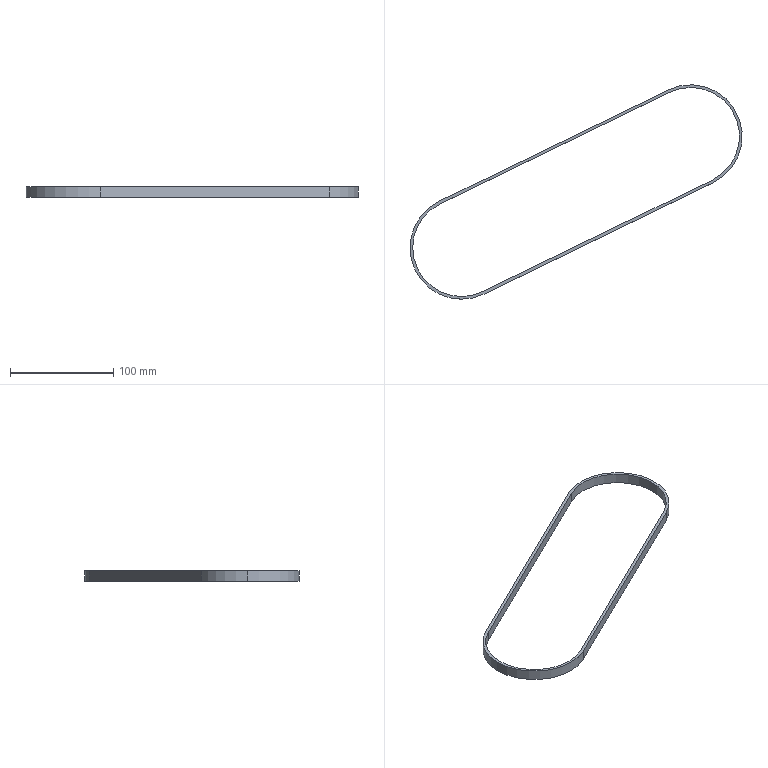Part | STEP file | Belt 1-18^ twist assembly SGN-4 | 1 solid | 12 faces | box 321.782 x 207.752 x 10 mm | volume 20933 mm3 | cylinder 6 | plane 6 | commonest cylinder face diameters 94.53 x3 99.77 x3
STEP:
#1=CARTESIAN_POINT('',(0.,0.,0.));
#2=DIRECTION('',(0.,0.,1.));
#3=DIRECTION('',(1.,0.,0.));
#4=AXIS2_PLACEMENT_3D('',#1,#2,#3);
#5=CARTESIAN_POINT('',(-141.649,-4.675,10.));
#6=VERTEX_POINT('',#5);
#7=CARTESIAN_POINT('',(-141.649,-4.675,0.));
#8=VERTEX_POINT('',#7);
#9=CARTESIAN_POINT('',(-141.649,-4.675,10.));
#10=DIRECTION('',(0.,0.,-1.));
#11=VECTOR('',#10,1.);
#12=LINE('',#9,#11);
#13=CARTESIAN_POINT('',(-120.976,-47.179,10.));
#14=DIRECTION('',(0.,0.,-1.));
#15=DIRECTION('',(-1.,0.,0.));
#16=AXIS2_PLACEMENT_3D('',#13,#14,#15);
#17=CYLINDRICAL_SURFACE('',#16,47.265);
#18=CARTESIAN_POINT('',(1.118,0.));
#19=DIRECTION('',(0.,1.));
#20=VECTOR('',#19,1.);
#21=LINE('',#18,#20);
#22=(GEOMETRIC_REPRESENTATION_CONTEXT(2)PARAMETRIC_REPRESENTATION_CONTEXT()REPRESENTATION_CONTEXT('',''));
#23=DEFINITIONAL_REPRESENTATION('',(#21),#22);
#24=PCURVE('',#17,#23);
#25=CARTESIAN_POINT('',(-141.649,-4.675,10.));
#26=DIRECTION('',(0.4374,-0.8993,0.));
#27=DIRECTION('',(0.8993,0.4374,0.));
#28=AXIS2_PLACEMENT_3D('',#25,#26,#27);
#29=PLANE('',#28);
#30=CARTESIAN_POINT('',(0.,0.));
#31=DIRECTION('',(0.,-1.));
#32=VECTOR('',#31,1.);
#33=LINE('',#30,#32);
#34=(GEOMETRIC_REPRESENTATION_CONTEXT(2)PARAMETRIC_REPRESENTATION_CONTEXT()REPRESENTATION_CONTEXT('',''));
#35=DEFINITIONAL_REPRESENTATION('',(#33),#34);
#36=PCURVE('',#29,#35);
#37=SURFACE_CURVE('',#12,(#24,#36),.PCURVE_S1.);
#38=EDGE_CURVE('',#6,#8,#37,.T.);
#39=ORIENTED_EDGE('',*,*,#38,.T.);
#40=CARTESIAN_POINT('',(-168.241,-47.179,0.));
#41=VERTEX_POINT('',#40);
#42=CARTESIAN_POINT('',(-120.976,-47.179,0.));
#43=DIRECTION('',(0.,0.,1.));
#44=DIRECTION('',(-1.,0.,0.));
#45=AXIS2_PLACEMENT_3D('',#42,#43,#44);
#46=CIRCLE('',#45,47.265);
#47=CARTESIAN_POINT('',(6.283,10.));
#48=DIRECTION('',(-1.,0.));
#49=VECTOR('',#48,1.);
#50=LINE('',#47,#49);
#51=(GEOMETRIC_REPRESENTATION_CONTEXT(2)PARAMETRIC_REPRESENTATION_CONTEXT()REPRESENTATION_CONTEXT('',''));
#52=DEFINITIONAL_REPRESENTATION('',(#50),#51);
#53=PCURVE('',#17,#52);
#54=CARTESIAN_POINT('',(-120.976,-47.179,0.));
#55=DIRECTION('',(0.,0.,-1.));
#56=DIRECTION('',(-1.,0.,0.));
#57=AXIS2_PLACEMENT_3D('',#54,#55,#56);
#58=PLANE('',#57);
#59=CARTESIAN_POINT('',(47.265,0.));
#60=CARTESIAN_POINT('',(47.265,-81.865));
#61=CARTESIAN_POINT('',(-23.633,-40.933));
#62=CARTESIAN_POINT('',(-94.53,0.));
#63=CARTESIAN_POINT('',(-23.633,40.933));
#64=CARTESIAN_POINT('',(47.265,81.865));
#65=CARTESIAN_POINT('',(47.265,0.));
#66=(BOUNDED_CURVE()B_SPLINE_CURVE(2,(#59,#60,#61,#62,#63,#64,#65),.UNSPECIFIED.,.T.,.F.)B_SPLINE_CURVE_WITH_KNOTS((1,2,2,2,2,1),(-2.094,0.,2.094,4.189,6.283,8.378),.UNSPECIFIED.)CURVE()GEOMETRIC_REPRESENTATION_ITEM()RATIONAL_B_SPLINE_CURVE((1.,0.5,1.,0.5,1.,0.5,1.))REPRESENTATION_ITEM(''));
#67=(GEOMETRIC_REPRESENTATION_CONTEXT(2)PARAMETRIC_REPRESENTATION_CONTEXT()REPRESENTATION_CONTEXT('',''));
#68=DEFINITIONAL_REPRESENTATION('',(#66),#67);
#69=PCURVE('',#58,#68);
#70=SURFACE_CURVE('',#46,(#53,#69),.PCURVE_S1.);
#71=EDGE_CURVE('',#8,#41,#70,.T.);
#72=ORIENTED_EDGE('',*,*,#71,.T.);
#73=CARTESIAN_POINT('',(-168.241,-47.179,10.));
#74=VERTEX_POINT('',#73);
#75=CARTESIAN_POINT('',(-168.241,-47.179,10.));
#76=DIRECTION('',(0.,0.,-1.));
#77=VECTOR('',#76,1.);
#78=LINE('',#75,#77);
#79=CARTESIAN_POINT('',(0.,0.));
#80=DIRECTION('',(0.,1.));
#81=VECTOR('',#80,1.);
#82=LINE('',#79,#81);
#83=(GEOMETRIC_REPRESENTATION_CONTEXT(2)PARAMETRIC_REPRESENTATION_CONTEXT()REPRESENTATION_CONTEXT('',''));
#84=DEFINITIONAL_REPRESENTATION('',(#82),#83);
#85=PCURVE('',#17,#84);
#86=CARTESIAN_POINT('',(-120.976,-47.179,10.));
#87=DIRECTION('',(0.,0.,-1.));
#88=DIRECTION('',(-1.,0.,0.));
#89=AXIS2_PLACEMENT_3D('',#86,#87,#88);
#90=CYLINDRICAL_SURFACE('',#89,47.265);
#91=CARTESIAN_POINT('',(6.283,0.));
#92=DIRECTION('',(0.,1.));
#93=VECTOR('',#92,1.);
#94=LINE('',#91,#93);
#95=(GEOMETRIC_REPRESENTATION_CONTEXT(2)PARAMETRIC_REPRESENTATION_CONTEXT()REPRESENTATION_CONTEXT('',''));
#96=DEFINITIONAL_REPRESENTATION('',(#94),#95);
#97=PCURVE('',#90,#96);
#98=SURFACE_CURVE('',#78,(#85,#97),.PCURVE_S1.);
#99=EDGE_CURVE('',#74,#41,#98,.T.);
#100=ORIENTED_EDGE('',*,*,#99,.F.);
#101=CARTESIAN_POINT('',(-120.976,-47.179,10.));
#102=DIRECTION('',(0.,0.,1.));
#103=DIRECTION('',(-1.,0.,0.));
#104=AXIS2_PLACEMENT_3D('',#101,#102,#103);
#105=CIRCLE('',#104,47.265);
#106=CARTESIAN_POINT('',(6.283,0.));
#107=DIRECTION('',(-1.,0.));
#108=VECTOR('',#107,1.);
#109=LINE('',#106,#108);
#110=(GEOMETRIC_REPRESENTATION_CONTEXT(2)PARAMETRIC_REPRESENTATION_CONTEXT()REPRESENTATION_CONTEXT('',''));
#111=DEFINITIONAL_REPRESENTATION('',(#109),#110);
#112=PCURVE('',#17,#111);
#113=CARTESIAN_POINT('',(-120.976,-47.179,10.));
#114=DIRECTION('',(0.,0.,-1.));
#115=DIRECTION('',(-1.,0.,0.));
#116=AXIS2_PLACEMENT_3D('',#113,#114,#115);
#117=PLANE('',#116);
#118=CARTESIAN_POINT('',(47.265,0.));
#119=CARTESIAN_POINT('',(47.265,-81.865));
#120=CARTESIAN_POINT('',(-23.633,-40.933));
#121=CARTESIAN_POINT('',(-94.53,0.));
#122=CARTESIAN_POINT('',(-23.633,40.933));
#123=CARTESIAN_POINT('',(47.265,81.865));
#124=CARTESIAN_POINT('',(47.265,0.));
#125=(BOUNDED_CURVE()B_SPLINE_CURVE(2,(#118,#119,#120,#121,#122,#123,#124),.UNSPECIFIED.,.T.,.F.)B_SPLINE_CURVE_WITH_KNOTS((1,2,2,2,2,1),(-2.094,0.,2.094,4.189,6.283,8.378),.UNSPECIFIED.)CURVE()GEOMETRIC_REPRESENTATION_ITEM()RATIONAL_B_SPLINE_CURVE((1.,0.5,1.,0.5,1.,0.5,1.))REPRESENTATION_ITEM(''));
#126=(GEOMETRIC_REPRESENTATION_CONTEXT(2)PARAMETRIC_REPRESENTATION_CONTEXT()REPRESENTATION_CONTEXT('',''));
#127=DEFINITIONAL_REPRESENTATION('',(#125),#126);
#128=PCURVE('',#117,#127);
#129=SURFACE_CURVE('',#105,(#112,#128),.PCURVE_S1.);
#130=EDGE_CURVE('',#6,#74,#129,.T.);
#131=ORIENTED_EDGE('',*,*,#130,.F.);
#132=EDGE_LOOP('',(#39,#72,#100,#131));
#133=FACE_BOUND('',#132,.F.);
#134=ADVANCED_FACE('',(#133),#17,.F.);
#135=CARTESIAN_POINT('',(-170.861,-47.179,10.));
#136=VERTEX_POINT('',#135);
#137=CARTESIAN_POINT('',(-99.156,-92.039,10.));
#138=VERTEX_POINT('',#137);
#139=CARTESIAN_POINT('',(-120.976,-47.179,10.));
#140=DIRECTION('',(0.,0.,1.));
#141=DIRECTION('',(-1.,0.,0.));
#142=AXIS2_PLACEMENT_3D('',#139,#140,#141);
#143=CIRCLE('',#142,49.885);
#144=CARTESIAN_POINT('',(-120.976,-47.179,10.));
#145=DIRECTION('',(0.,0.,-1.));
#146=DIRECTION('',(-1.,0.,0.));
#147=AXIS2_PLACEMENT_3D('',#144,#145,#146);
#148=CYLINDRICAL_SURFACE('',#147,49.885);
#149=CARTESIAN_POINT('',(6.283,0.));
#150=DIRECTION('',(-1.,0.));
#151=VECTOR('',#150,1.);
#152=LINE('',#149,#151);
#153=(GEOMETRIC_REPRESENTATION_CONTEXT(2)PARAMETRIC_REPRESENTATION_CONTEXT()REPRESENTATION_CONTEXT('',''));
#154=DEFINITIONAL_REPRESENTATION('',(#152),#153);
#155=PCURVE('',#148,#154);
#156=CARTESIAN_POINT('',(49.885,0.));
#157=CARTESIAN_POINT('',(49.885,-86.403));
#158=CARTESIAN_POINT('',(-24.942,-43.202));
#159=CARTESIAN_POINT('',(-99.77,0.));
#160=CARTESIAN_POINT('',(-24.942,43.202));
#161=CARTESIAN_POINT('',(49.885,86.403));
#162=CARTESIAN_POINT('',(49.885,0.));
#163=(BOUNDED_CURVE()B_SPLINE_CURVE(2,(#156,#157,#158,#159,#160,#161,#162),.UNSPECIFIED.,.T.,.F.)B_SPLINE_CURVE_WITH_KNOTS((1,2,2,2,2,1),(-2.094,0.,2.094,4.189,6.283,8.378),.UNSPECIFIED.)CURVE()GEOMETRIC_REPRESENTATION_ITEM()RATIONAL_B_SPLINE_CURVE((1.,0.5,1.,0.5,1.,0.5,1.))REPRESENTATION_ITEM(''));
#164=(GEOMETRIC_REPRESENTATION_CONTEXT(2)PARAMETRIC_REPRESENTATION_CONTEXT()REPRESENTATION_CONTEXT('',''));
#165=DEFINITIONAL_REPRESENTATION('',(#163),#164);
#166=PCURVE('',#117,#165);
#167=SURFACE_CURVE('',#143,(#155,#166),.PCURVE_S1.);
#168=EDGE_CURVE('',#136,#138,#167,.T.);
#169=ORIENTED_EDGE('',*,*,#168,.F.);
#170=CARTESIAN_POINT('',(-170.861,-47.179,0.));
#171=VERTEX_POINT('',#170);
#172=CARTESIAN_POINT('',(-170.861,-47.179,10.));
#173=DIRECTION('',(0.,0.,-1.));
#174=VECTOR('',#173,1.);
#175=LINE('',#172,#174);
#176=CARTESIAN_POINT('',(6.283,0.));
#177=DIRECTION('',(0.,1.));
#178=VECTOR('',#177,1.);
#179=LINE('',#176,#178);
#180=(GEOMETRIC_REPRESENTATION_CONTEXT(2)PARAMETRIC_REPRESENTATION_CONTEXT()REPRESENTATION_CONTEXT('',''));
#181=DEFINITIONAL_REPRESENTATION('',(#179),#180);
#182=PCURVE('',#148,#181);
#183=CARTESIAN_POINT('',(-120.976,-47.179,10.));
#184=DIRECTION('',(0.,0.,-1.));
#185=DIRECTION('',(-1.,0.,0.));
#186=AXIS2_PLACEMENT_3D('',#183,#184,#185);
#187=CYLINDRICAL_SURFACE('',#186,49.885);
#188=CARTESIAN_POINT('',(0.,0.));
#189=DIRECTION('',(0.,1.));
#190=VECTOR('',#189,1.);
#191=LINE('',#188,#190);
#192=(GEOMETRIC_REPRESENTATION_CONTEXT(2)PARAMETRIC_REPRESENTATION_CONTEXT()REPRESENTATION_CONTEXT('',''));
#193=DEFINITIONAL_REPRESENTATION('',(#191),#192);
#194=PCURVE('',#187,#193);
#195=SURFACE_CURVE('',#175,(#182,#194),.PCURVE_S1.);
#196=EDGE_CURVE('',#136,#171,#195,.T.);
#197=ORIENTED_EDGE('',*,*,#196,.T.);
#198=CARTESIAN_POINT('',(-99.156,-92.039,0.));
#199=VERTEX_POINT('',#198);
#200=CARTESIAN_POINT('',(-120.976,-47.179,0.));
#201=DIRECTION('',(0.,0.,1.));
#202=DIRECTION('',(-1.,0.,0.));
#203=AXIS2_PLACEMENT_3D('',#200,#201,#202);
#204=CIRCLE('',#203,49.885);
#205=CARTESIAN_POINT('',(6.283,10.));
#206=DIRECTION('',(-1.,0.));
#207=VECTOR('',#206,1.);
#208=LINE('',#205,#207);
#209=(GEOMETRIC_REPRESENTATION_CONTEXT(2)PARAMETRIC_REPRESENTATION_CONTEXT()REPRESENTATION_CONTEXT('',''));
#210=DEFINITIONAL_REPRESENTATION('',(#208),#209);
#211=PCURVE('',#148,#210);
#212=CARTESIAN_POINT('',(49.885,0.));
#213=CARTESIAN_POINT('',(49.885,-86.403));
#214=CARTESIAN_POINT('',(-24.942,-43.202));
#215=CARTESIAN_POINT('',(-99.77,0.));
#216=CARTESIAN_POINT('',(-24.942,43.202));
#217=CARTESIAN_POINT('',(49.885,86.403));
#218=CARTESIAN_POINT('',(49.885,0.));
#219=(BOUNDED_CURVE()B_SPLINE_CURVE(2,(#212,#213,#214,#215,#216,#217,#218),.UNSPECIFIED.,.T.,.F.)B_SPLINE_CURVE_WITH_KNOTS((1,2,2,2,2,1),(-2.094,0.,2.094,4.189,6.283,8.378),.UNSPECIFIED.)CURVE()GEOMETRIC_REPRESENTATION_ITEM()RATIONAL_B_SPLINE_CURVE((1.,0.5,1.,0.5,1.,0.5,1.))REPRESENTATION_ITEM(''));
#220=(GEOMETRIC_REPRESENTATION_CONTEXT(2)PARAMETRIC_REPRESENTATION_CONTEXT()REPRESENTATION_CONTEXT('',''));
#221=DEFINITIONAL_REPRESENTATION('',(#219),#220);
#222=PCURVE('',#58,#221);
#223=SURFACE_CURVE('',#204,(#211,#222),.PCURVE_S1.);
#224=EDGE_CURVE('',#171,#199,#223,.T.);
#225=ORIENTED_EDGE('',*,*,#224,.T.);
#226=CARTESIAN_POINT('',(-99.156,-92.039,10.));
#227=DIRECTION('',(0.,0.,-1.));
#228=VECTOR('',#227,1.);
#229=LINE('',#226,#228);
#230=CARTESIAN_POINT('',(4.26,0.));
#231=DIRECTION('',(0.,1.));
#232=VECTOR('',#231,1.);
#233=LINE('',#230,#232);
#234=(GEOMETRIC_REPRESENTATION_CONTEXT(2)PARAMETRIC_REPRESENTATION_CONTEXT()REPRESENTATION_CONTEXT('',''));
#235=DEFINITIONAL_REPRESENTATION('',(#233),#234);
#236=PCURVE('',#148,#235);
#237=CARTESIAN_POINT('',(-99.156,-92.039,10.));
#238=DIRECTION('',(-0.4374,0.8993,0.));
#239=DIRECTION('',(-0.8993,-0.4374,0.));
#240=AXIS2_PLACEMENT_3D('',#237,#238,#239);
#241=PLANE('',#240);
#242=CARTESIAN_POINT('',(0.,0.));
#243=DIRECTION('',(0.,-1.));
#244=VECTOR('',#243,1.);
#245=LINE('',#242,#244);
#246=(GEOMETRIC_REPRESENTATION_CONTEXT(2)PARAMETRIC_REPRESENTATION_CONTEXT()REPRESENTATION_CONTEXT('',''));
#247=DEFINITIONAL_REPRESENTATION('',(#245),#246);
#248=PCURVE('',#241,#247);
#249=SURFACE_CURVE('',#229,(#236,#248),.PCURVE_S1.);
#250=EDGE_CURVE('',#138,#199,#249,.T.);
#251=ORIENTED_EDGE('',*,*,#250,.F.);
#252=EDGE_LOOP('',(#169,#197,#225,#251));
#253=FACE_BOUND('',#252,.T.);
#254=ADVANCED_FACE('',(#253),#148,.T.);
#255=CARTESIAN_POINT('',(-142.795,-2.318,10.));
#256=VERTEX_POINT('',#255);
#257=CARTESIAN_POINT('',(-120.976,-47.179,10.));
#258=DIRECTION('',(0.,0.,1.));
#259=DIRECTION('',(-1.,0.,0.));
#260=AXIS2_PLACEMENT_3D('',#257,#258,#259);
#261=CIRCLE('',#260,49.885);
#262=CARTESIAN_POINT('',(49.885,0.));
#263=CARTESIAN_POINT('',(49.885,-86.403));
#264=CARTESIAN_POINT('',(-24.942,-43.202));
#265=CARTESIAN_POINT('',(-99.77,0.));
#266=CARTESIAN_POINT('',(-24.942,43.202));
#267=CARTESIAN_POINT('',(49.885,86.403));
#268=CARTESIAN_POINT('',(49.885,0.));
#269=(BOUNDED_CURVE()B_SPLINE_CURVE(2,(#262,#263,#264,#265,#266,#267,#268),.UNSPECIFIED.,.T.,.F.)B_SPLINE_CURVE_WITH_KNOTS((1,2,2,2,2,1),(-2.094,0.,2.094,4.189,6.283,8.378),.UNSPECIFIED.)CURVE()GEOMETRIC_REPRESENTATION_ITEM()RATIONAL_B_SPLINE_CURVE((1.,0.5,1.,0.5,1.,0.5,1.))REPRESENTATION_ITEM(''));
#270=(GEOMETRIC_REPRESENTATION_CONTEXT(2)PARAMETRIC_REPRESENTATION_CONTEXT()REPRESENTATION_CONTEXT('',''));
#271=DEFINITIONAL_REPRESENTATION('',(#269),#270);
#272=PCURVE('',#117,#271);
#273=CARTESIAN_POINT('',(6.283,0.));
#274=DIRECTION('',(-1.,0.));
#275=VECTOR('',#274,1.);
#276=LINE('',#273,#275);
#277=(GEOMETRIC_REPRESENTATION_CONTEXT(2)PARAMETRIC_REPRESENTATION_CONTEXT()REPRESENTATION_CONTEXT('',''));
#278=DEFINITIONAL_REPRESENTATION('',(#276),#277);
#279=PCURVE('',#187,#278);
#280=SURFACE_CURVE('',#261,(#272,#279),.PCURVE_S1.);
#281=EDGE_CURVE('',#256,#136,#280,.T.);
#282=ORIENTED_EDGE('',*,*,#281,.T.);
#283=ORIENTED_EDGE('',*,*,#168,.T.);
#284=CARTESIAN_POINT('',(122.856,15.944,10.));
#285=VERTEX_POINT('',#284);
#286=CARTESIAN_POINT('',(-99.156,-92.039,10.));
#287=DIRECTION('',(0.8993,0.4374,0.));
#288=VECTOR('',#287,1.);
#289=LINE('',#286,#288);
#290=CARTESIAN_POINT('',(-21.819,-44.86));
#291=DIRECTION('',(-0.8993,0.4374));
#292=VECTOR('',#291,1.);
#293=LINE('',#290,#292);
#294=(GEOMETRIC_REPRESENTATION_CONTEXT(2)PARAMETRIC_REPRESENTATION_CONTEXT()REPRESENTATION_CONTEXT('',''));
#295=DEFINITIONAL_REPRESENTATION('',(#293),#294);
#296=PCURVE('',#117,#295);
#297=CARTESIAN_POINT('',(0.,0.));
#298=DIRECTION('',(-1.,0.));
#299=VECTOR('',#298,1.);
#300=LINE('',#297,#299);
#301=(GEOMETRIC_REPRESENTATION_CONTEXT(2)PARAMETRIC_REPRESENTATION_CONTEXT()REPRESENTATION_CONTEXT('',''));
#302=DEFINITIONAL_REPRESENTATION('',(#300),#301);
#303=PCURVE('',#241,#302);
#304=SURFACE_CURVE('',#289,(#296,#303),.PCURVE_S1.);
#305=EDGE_CURVE('',#138,#285,#304,.T.);
#306=ORIENTED_EDGE('',*,*,#305,.T.);
#307=CARTESIAN_POINT('',(79.218,105.664,10.));
#308=VERTEX_POINT('',#307);
#309=CARTESIAN_POINT('',(101.037,60.804,10.));
#310=DIRECTION('',(0.,0.,1.));
#311=DIRECTION('',(-1.,0.,0.));
#312=AXIS2_PLACEMENT_3D('',#309,#310,#311);
#313=CIRCLE('',#312,49.885);
#314=CARTESIAN_POINT('',(-172.127,107.982));
#315=CARTESIAN_POINT('',(-172.127,21.579));
#316=CARTESIAN_POINT('',(-246.955,64.781));
#317=CARTESIAN_POINT('',(-321.782,107.982));
#318=CARTESIAN_POINT('',(-246.955,151.184));
#319=CARTESIAN_POINT('',(-172.127,194.386));
#320=CARTESIAN_POINT('',(-172.127,107.982));
#321=(BOUNDED_CURVE()B_SPLINE_CURVE(2,(#314,#315,#316,#317,#318,#319,#320),.UNSPECIFIED.,.T.,.F.)B_SPLINE_CURVE_WITH_KNOTS((1,2,2,2,2,1),(-2.094,0.,2.094,4.189,6.283,8.378),.UNSPECIFIED.)CURVE()GEOMETRIC_REPRESENTATION_ITEM()RATIONAL_B_SPLINE_CURVE((1.,0.5,1.,0.5,1.,0.5,1.))REPRESENTATION_ITEM(''));
#322=(GEOMETRIC_REPRESENTATION_CONTEXT(2)PARAMETRIC_REPRESENTATION_CONTEXT()REPRESENTATION_CONTEXT('',''));
#323=DEFINITIONAL_REPRESENTATION('',(#321),#322);
#324=PCURVE('',#117,#323);
#325=CARTESIAN_POINT('',(101.037,60.804,10.));
#326=DIRECTION('',(0.,0.,-1.));
#327=DIRECTION('',(-1.,0.,0.));
#328=AXIS2_PLACEMENT_3D('',#325,#326,#327);
#329=CYLINDRICAL_SURFACE('',#328,49.885);
#330=CARTESIAN_POINT('',(6.283,0.));
#331=DIRECTION('',(-1.,0.));
#332=VECTOR('',#331,1.);
#333=LINE('',#330,#332);
#334=(GEOMETRIC_REPRESENTATION_CONTEXT(2)PARAMETRIC_REPRESENTATION_CONTEXT()REPRESENTATION_CONTEXT('',''));
#335=DEFINITIONAL_REPRESENTATION('',(#333),#334);
#336=PCURVE('',#329,#335);
#337=SURFACE_CURVE('',#313,(#324,#336),.PCURVE_S1.);
#338=EDGE_CURVE('',#285,#308,#337,.T.);
#339=ORIENTED_EDGE('',*,*,#338,.T.);
#340=CARTESIAN_POINT('',(-142.795,-2.318,10.));
#341=DIRECTION('',(-0.8993,-0.4374,0.));
#342=VECTOR('',#341,1.);
#343=LINE('',#340,#342);
#344=CARTESIAN_POINT('',(21.819,44.86));
#345=DIRECTION('',(0.8993,-0.4374));
#346=VECTOR('',#345,1.);
#347=LINE('',#344,#346);
#348=(GEOMETRIC_REPRESENTATION_CONTEXT(2)PARAMETRIC_REPRESENTATION_CONTEXT()REPRESENTATION_CONTEXT('',''));
#349=DEFINITIONAL_REPRESENTATION('',(#347),#348);
#350=PCURVE('',#117,#349);
#351=CARTESIAN_POINT('',(-142.795,-2.318,10.));
#352=DIRECTION('',(0.4374,-0.8993,0.));
#353=DIRECTION('',(0.8993,0.4374,0.));
#354=AXIS2_PLACEMENT_3D('',#351,#352,#353);
#355=PLANE('',#354);
#356=CARTESIAN_POINT('',(0.,0.));
#357=DIRECTION('',(-1.,0.));
#358=VECTOR('',#357,1.);
#359=LINE('',#356,#358);
#360=(GEOMETRIC_REPRESENTATION_CONTEXT(2)PARAMETRIC_REPRESENTATION_CONTEXT()REPRESENTATION_CONTEXT('',''));
#361=DEFINITIONAL_REPRESENTATION('',(#359),#360);
#362=PCURVE('',#355,#361);
#363=SURFACE_CURVE('',#343,(#350,#362),.PCURVE_S1.);
#364=EDGE_CURVE('',#308,#256,#363,.T.);
#365=ORIENTED_EDGE('',*,*,#364,.T.);
#366=EDGE_LOOP('',(#282,#283,#306,#339,#365));
#367=FACE_BOUND('',#366,.T.);
#368=ORIENTED_EDGE('',*,*,#130,.F.);
#369=CARTESIAN_POINT('',(80.364,103.308,10.));
#370=VERTEX_POINT('',#369);
#371=CARTESIAN_POINT('',(-141.649,-4.675,10.));
#372=DIRECTION('',(-0.8993,-0.4374,0.));
#373=VECTOR('',#372,1.);
#374=LINE('',#371,#373);
#375=CARTESIAN_POINT('',(20.673,42.504));
#376=DIRECTION('',(0.8993,-0.4374));
#377=VECTOR('',#376,1.);
#378=LINE('',#375,#377);
#379=(GEOMETRIC_REPRESENTATION_CONTEXT(2)PARAMETRIC_REPRESENTATION_CONTEXT()REPRESENTATION_CONTEXT('',''));
#380=DEFINITIONAL_REPRESENTATION('',(#378),#379);
#381=PCURVE('',#117,#380);
#382=CARTESIAN_POINT('',(0.,0.));
#383=DIRECTION('',(-1.,0.));
#384=VECTOR('',#383,1.);
#385=LINE('',#382,#384);
#386=(GEOMETRIC_REPRESENTATION_CONTEXT(2)PARAMETRIC_REPRESENTATION_CONTEXT()REPRESENTATION_CONTEXT('',''));
#387=DEFINITIONAL_REPRESENTATION('',(#385),#386);
#388=PCURVE('',#29,#387);
#389=SURFACE_CURVE('',#374,(#381,#388),.PCURVE_S1.);
#390=EDGE_CURVE('',#370,#6,#389,.T.);
#391=ORIENTED_EDGE('',*,*,#390,.F.);
#392=CARTESIAN_POINT('',(121.71,18.3,10.));
#393=VERTEX_POINT('',#392);
#394=CARTESIAN_POINT('',(101.037,60.804,10.));
#395=DIRECTION('',(0.,0.,1.));
#396=DIRECTION('',(-1.,0.,0.));
#397=AXIS2_PLACEMENT_3D('',#394,#395,#396);
#398=CIRCLE('',#397,47.265);
#399=CARTESIAN_POINT('',(-174.747,107.982));
#400=CARTESIAN_POINT('',(-174.747,26.117));
#401=CARTESIAN_POINT('',(-245.645,67.05));
#402=CARTESIAN_POINT('',(-316.542,107.982));
#403=CARTESIAN_POINT('',(-245.645,148.915));
#404=CARTESIAN_POINT('',(-174.747,189.848));
#405=CARTESIAN_POINT('',(-174.747,107.982));
#406=(BOUNDED_CURVE()B_SPLINE_CURVE(2,(#399,#400,#401,#402,#403,#404,#405),.UNSPECIFIED.,.T.,.F.)B_SPLINE_CURVE_WITH_KNOTS((1,2,2,2,2,1),(-2.094,0.,2.094,4.189,6.283,8.378),.UNSPECIFIED.)CURVE()GEOMETRIC_REPRESENTATION_ITEM()RATIONAL_B_SPLINE_CURVE((1.,0.5,1.,0.5,1.,0.5,1.))REPRESENTATION_ITEM(''));
#407=(GEOMETRIC_REPRESENTATION_CONTEXT(2)PARAMETRIC_REPRESENTATION_CONTEXT()REPRESENTATION_CONTEXT('',''));
#408=DEFINITIONAL_REPRESENTATION('',(#406),#407);
#409=PCURVE('',#117,#408);
#410=CARTESIAN_POINT('',(101.037,60.804,10.));
#411=DIRECTION('',(0.,0.,-1.));
#412=DIRECTION('',(-1.,0.,0.));
#413=AXIS2_PLACEMENT_3D('',#410,#411,#412);
#414=CYLINDRICAL_SURFACE('',#413,47.265);
#415=CARTESIAN_POINT('',(6.283,0.));
#416=DIRECTION('',(-1.,0.));
#417=VECTOR('',#416,1.);
#418=LINE('',#415,#417);
#419=(GEOMETRIC_REPRESENTATION_CONTEXT(2)PARAMETRIC_REPRESENTATION_CONTEXT()REPRESENTATION_CONTEXT('',''));
#420=DEFINITIONAL_REPRESENTATION('',(#418),#419);
#421=PCURVE('',#414,#420);
#422=SURFACE_CURVE('',#398,(#409,#421),.PCURVE_S1.);
#423=EDGE_CURVE('',#393,#370,#422,.T.);
#424=ORIENTED_EDGE('',*,*,#423,.F.);
#425=CARTESIAN_POINT('',(-100.302,-89.683,10.));
#426=VERTEX_POINT('',#425);
#427=CARTESIAN_POINT('',(121.71,18.3,10.));
#428=DIRECTION('',(0.8993,0.4374,0.));
#429=VECTOR('',#428,1.);
#430=LINE('',#427,#429);
#431=CARTESIAN_POINT('',(-242.686,65.478));
#432=DIRECTION('',(-0.8993,0.4374));
#433=VECTOR('',#432,1.);
#434=LINE('',#431,#433);
#435=(GEOMETRIC_REPRESENTATION_CONTEXT(2)PARAMETRIC_REPRESENTATION_CONTEXT()REPRESENTATION_CONTEXT('',''));
#436=DEFINITIONAL_REPRESENTATION('',(#434),#435);
#437=PCURVE('',#117,#436);
#438=CARTESIAN_POINT('',(121.71,18.3,10.));
#439=DIRECTION('',(-0.4374,0.8993,0.));
#440=DIRECTION('',(-0.8993,-0.4374,0.));
#441=AXIS2_PLACEMENT_3D('',#438,#439,#440);
#442=PLANE('',#441);
#443=CARTESIAN_POINT('',(0.,0.));
#444=DIRECTION('',(-1.,0.));
#445=VECTOR('',#444,1.);
#446=LINE('',#443,#445);
#447=(GEOMETRIC_REPRESENTATION_CONTEXT(2)PARAMETRIC_REPRESENTATION_CONTEXT()REPRESENTATION_CONTEXT('',''));
#448=DEFINITIONAL_REPRESENTATION('',(#446),#447);
#449=PCURVE('',#442,#448);
#450=SURFACE_CURVE('',#430,(#437,#449),.PCURVE_S1.);
#451=EDGE_CURVE('',#426,#393,#450,.T.);
#452=ORIENTED_EDGE('',*,*,#451,.F.);
#453=CARTESIAN_POINT('',(-120.976,-47.179,10.));
#454=DIRECTION('',(0.,0.,1.));
#455=DIRECTION('',(-1.,0.,0.));
#456=AXIS2_PLACEMENT_3D('',#453,#454,#455);
#457=CIRCLE('',#456,47.265);
#458=CARTESIAN_POINT('',(47.265,0.));
#459=CARTESIAN_POINT('',(47.265,-81.865));
#460=CARTESIAN_POINT('',(-23.633,-40.933));
#461=CARTESIAN_POINT('',(-94.53,0.));
#462=CARTESIAN_POINT('',(-23.633,40.933));
#463=CARTESIAN_POINT('',(47.265,81.865));
#464=CARTESIAN_POINT('',(47.265,0.));
#465=(BOUNDED_CURVE()B_SPLINE_CURVE(2,(#458,#459,#460,#461,#462,#463,#464),.UNSPECIFIED.,.T.,.F.)B_SPLINE_CURVE_WITH_KNOTS((1,2,2,2,2,1),(-2.094,0.,2.094,4.189,6.283,8.378),.UNSPECIFIED.)CURVE()GEOMETRIC_REPRESENTATION_ITEM()RATIONAL_B_SPLINE_CURVE((1.,0.5,1.,0.5,1.,0.5,1.))REPRESENTATION_ITEM(''));
#466=(GEOMETRIC_REPRESENTATION_CONTEXT(2)PARAMETRIC_REPRESENTATION_CONTEXT()REPRESENTATION_CONTEXT('',''));
#467=DEFINITIONAL_REPRESENTATION('',(#465),#466);
#468=PCURVE('',#117,#467);
#469=CARTESIAN_POINT('',(6.283,0.));
#470=DIRECTION('',(-1.,0.));
#471=VECTOR('',#470,1.);
#472=LINE('',#469,#471);
#473=(GEOMETRIC_REPRESENTATION_CONTEXT(2)PARAMETRIC_REPRESENTATION_CONTEXT()REPRESENTATION_CONTEXT('',''));
#474=DEFINITIONAL_REPRESENTATION('',(#472),#473);
#475=PCURVE('',#90,#474);
#476=SURFACE_CURVE('',#457,(#468,#475),.PCURVE_S1.);
#477=EDGE_CURVE('',#74,#426,#476,.T.);
#478=ORIENTED_EDGE('',*,*,#477,.F.);
#479=EDGE_LOOP('',(#368,#391,#424,#452,#478));
#480=FACE_BOUND('',#479,.T.);
#481=ADVANCED_FACE('',(#367,#480),#117,.F.);
#482=CARTESIAN_POINT('',(-142.795,-2.318,0.));
#483=VERTEX_POINT('',#482);
#484=CARTESIAN_POINT('',(-120.976,-47.179,0.));
#485=DIRECTION('',(0.,0.,1.));
#486=DIRECTION('',(-1.,0.,0.));
#487=AXIS2_PLACEMENT_3D('',#484,#485,#486);
#488=CIRCLE('',#487,49.885);
#489=CARTESIAN_POINT('',(49.885,0.));
#490=CARTESIAN_POINT('',(49.885,-86.403));
#491=CARTESIAN_POINT('',(-24.942,-43.202));
#492=CARTESIAN_POINT('',(-99.77,0.));
#493=CARTESIAN_POINT('',(-24.942,43.202));
#494=CARTESIAN_POINT('',(49.885,86.403));
#495=CARTESIAN_POINT('',(49.885,0.));
#496=(BOUNDED_CURVE()B_SPLINE_CURVE(2,(#489,#490,#491,#492,#493,#494,#495),.UNSPECIFIED.,.T.,.F.)B_SPLINE_CURVE_WITH_KNOTS((1,2,2,2,2,1),(-2.094,0.,2.094,4.189,6.283,8.378),.UNSPECIFIED.)CURVE()GEOMETRIC_REPRESENTATION_ITEM()RATIONAL_B_SPLINE_CURVE((1.,0.5,1.,0.5,1.,0.5,1.))REPRESENTATION_ITEM(''));
#497=(GEOMETRIC_REPRESENTATION_CONTEXT(2)PARAMETRIC_REPRESENTATION_CONTEXT()REPRESENTATION_CONTEXT('',''));
#498=DEFINITIONAL_REPRESENTATION('',(#496),#497);
#499=PCURVE('',#58,#498);
#500=CARTESIAN_POINT('',(6.283,10.));
#501=DIRECTION('',(-1.,0.));
#502=VECTOR('',#501,1.);
#503=LINE('',#500,#502);
#504=(GEOMETRIC_REPRESENTATION_CONTEXT(2)PARAMETRIC_REPRESENTATION_CONTEXT()REPRESENTATION_CONTEXT('',''));
#505=DEFINITIONAL_REPRESENTATION('',(#503),#504);
#506=PCURVE('',#187,#505);
#507=SURFACE_CURVE('',#488,(#499,#506),.PCURVE_S1.);
#508=EDGE_CURVE('',#483,#171,#507,.T.);
#509=ORIENTED_EDGE('',*,*,#508,.F.);
#510=CARTESIAN_POINT('',(79.218,105.664,0.));
#511=VERTEX_POINT('',#510);
#512=CARTESIAN_POINT('',(-142.795,-2.318,0.));
#513=DIRECTION('',(-0.8993,-0.4374,0.));
#514=VECTOR('',#513,1.);
#515=LINE('',#512,#514);
#516=CARTESIAN_POINT('',(21.819,44.86));
#517=DIRECTION('',(0.8993,-0.4374));
#518=VECTOR('',#517,1.);
#519=LINE('',#516,#518);
#520=(GEOMETRIC_REPRESENTATION_CONTEXT(2)PARAMETRIC_REPRESENTATION_CONTEXT()REPRESENTATION_CONTEXT('',''));
#521=DEFINITIONAL_REPRESENTATION('',(#519),#520);
#522=PCURVE('',#58,#521);
#523=CARTESIAN_POINT('',(0.,-10.));
#524=DIRECTION('',(-1.,0.));
#525=VECTOR('',#524,1.);
#526=LINE('',#523,#525);
#527=(GEOMETRIC_REPRESENTATION_CONTEXT(2)PARAMETRIC_REPRESENTATION_CONTEXT()REPRESENTATION_CONTEXT('',''));
#528=DEFINITIONAL_REPRESENTATION('',(#526),#527);
#529=PCURVE('',#355,#528);
#530=SURFACE_CURVE('',#515,(#522,#529),.PCURVE_S1.);
#531=EDGE_CURVE('',#511,#483,#530,.T.);
#532=ORIENTED_EDGE('',*,*,#531,.F.);
#533=CARTESIAN_POINT('',(122.856,15.944,0.));
#534=VERTEX_POINT('',#533);
#535=CARTESIAN_POINT('',(101.037,60.804,0.));
#536=DIRECTION('',(0.,0.,1.));
#537=DIRECTION('',(-1.,0.,0.));
#538=AXIS2_PLACEMENT_3D('',#535,#536,#537);
#539=CIRCLE('',#538,49.885);
#540=CARTESIAN_POINT('',(-172.127,107.982));
#541=CARTESIAN_POINT('',(-172.127,21.579));
#542=CARTESIAN_POINT('',(-246.955,64.781));
#543=CARTESIAN_POINT('',(-321.782,107.982));
#544=CARTESIAN_POINT('',(-246.955,151.184));
#545=CARTESIAN_POINT('',(-172.127,194.386));
#546=CARTESIAN_POINT('',(-172.127,107.982));
#547=(BOUNDED_CURVE()B_SPLINE_CURVE(2,(#540,#541,#542,#543,#544,#545,#546),.UNSPECIFIED.,.T.,.F.)B_SPLINE_CURVE_WITH_KNOTS((1,2,2,2,2,1),(-2.094,0.,2.094,4.189,6.283,8.378),.UNSPECIFIED.)CURVE()GEOMETRIC_REPRESENTATION_ITEM()RATIONAL_B_SPLINE_CURVE((1.,0.5,1.,0.5,1.,0.5,1.))REPRESENTATION_ITEM(''));
#548=(GEOMETRIC_REPRESENTATION_CONTEXT(2)PARAMETRIC_REPRESENTATION_CONTEXT()REPRESENTATION_CONTEXT('',''));
#549=DEFINITIONAL_REPRESENTATION('',(#547),#548);
#550=PCURVE('',#58,#549);
#551=CARTESIAN_POINT('',(6.283,10.));
#552=DIRECTION('',(-1.,0.));
#553=VECTOR('',#552,1.);
#554=LINE('',#551,#553);
#555=(GEOMETRIC_REPRESENTATION_CONTEXT(2)PARAMETRIC_REPRESENTATION_CONTEXT()REPRESENTATION_CONTEXT('',''));
#556=DEFINITIONAL_REPRESENTATION('',(#554),#555);
#557=PCURVE('',#329,#556);
#558=SURFACE_CURVE('',#539,(#550,#557),.PCURVE_S1.);
#559=EDGE_CURVE('',#534,#511,#558,.T.);
#560=ORIENTED_EDGE('',*,*,#559,.F.);
#561=CARTESIAN_POINT('',(-99.156,-92.039,0.));
#562=DIRECTION('',(0.8993,0.4374,0.));
#563=VECTOR('',#562,1.);
#564=LINE('',#561,#563);
#565=CARTESIAN_POINT('',(-21.819,-44.86));
#566=DIRECTION('',(-0.8993,0.4374));
#567=VECTOR('',#566,1.);
#568=LINE('',#565,#567);
#569=(GEOMETRIC_REPRESENTATION_CONTEXT(2)PARAMETRIC_REPRESENTATION_CONTEXT()REPRESENTATION_CONTEXT('',''));
#570=DEFINITIONAL_REPRESENTATION('',(#568),#569);
#571=PCURVE('',#58,#570);
#572=CARTESIAN_POINT('',(0.,-10.));
#573=DIRECTION('',(-1.,0.));
#574=VECTOR('',#573,1.);
#575=LINE('',#572,#574);
#576=(GEOMETRIC_REPRESENTATION_CONTEXT(2)PARAMETRIC_REPRESENTATION_CONTEXT()REPRESENTATION_CONTEXT('',''));
#577=DEFINITIONAL_REPRESENTATION('',(#575),#576);
#578=PCURVE('',#241,#577);
#579=SURFACE_CURVE('',#564,(#571,#578),.PCURVE_S1.);
#580=EDGE_CURVE('',#199,#534,#579,.T.);
#581=ORIENTED_EDGE('',*,*,#580,.F.);
#582=ORIENTED_EDGE('',*,*,#224,.F.);
#583=EDGE_LOOP('',(#509,#532,#560,#581,#582));
#584=FACE_BOUND('',#583,.T.);
#585=CARTESIAN_POINT('',(80.364,103.308,0.));
#586=VERTEX_POINT('',#585);
#587=CARTESIAN_POINT('',(-141.649,-4.675,0.));
#588=DIRECTION('',(-0.8993,-0.4374,0.));
#589=VECTOR('',#588,1.);
#590=LINE('',#587,#589);
#591=CARTESIAN_POINT('',(20.673,42.504));
#592=DIRECTION('',(0.8993,-0.4374));
#593=VECTOR('',#592,1.);
#594=LINE('',#591,#593);
#595=(GEOMETRIC_REPRESENTATION_CONTEXT(2)PARAMETRIC_REPRESENTATION_CONTEXT()REPRESENTATION_CONTEXT('',''));
#596=DEFINITIONAL_REPRESENTATION('',(#594),#595);
#597=PCURVE('',#58,#596);
#598=CARTESIAN_POINT('',(0.,-10.));
#599=DIRECTION('',(-1.,0.));
#600=VECTOR('',#599,1.);
#601=LINE('',#598,#600);
#602=(GEOMETRIC_REPRESENTATION_CONTEXT(2)PARAMETRIC_REPRESENTATION_CONTEXT()REPRESENTATION_CONTEXT('',''));
#603=DEFINITIONAL_REPRESENTATION('',(#601),#602);
#604=PCURVE('',#29,#603);
#605=SURFACE_CURVE('',#590,(#597,#604),.PCURVE_S1.);
#606=EDGE_CURVE('',#586,#8,#605,.T.);
#607=ORIENTED_EDGE('',*,*,#606,.T.);
#608=ORIENTED_EDGE('',*,*,#71,.T.);
#609=CARTESIAN_POINT('',(-100.302,-89.683,0.));
#610=VERTEX_POINT('',#609);
#611=CARTESIAN_POINT('',(-120.976,-47.179,0.));
#612=DIRECTION('',(0.,0.,1.));
#613=DIRECTION('',(-1.,0.,0.));
#614=AXIS2_PLACEMENT_3D('',#611,#612,#613);
#615=CIRCLE('',#614,47.265);
#616=CARTESIAN_POINT('',(47.265,0.));
#617=CARTESIAN_POINT('',(47.265,-81.865));
#618=CARTESIAN_POINT('',(-23.633,-40.933));
#619=CARTESIAN_POINT('',(-94.53,0.));
#620=CARTESIAN_POINT('',(-23.633,40.933));
#621=CARTESIAN_POINT('',(47.265,81.865));
#622=CARTESIAN_POINT('',(47.265,0.));
#623=(BOUNDED_CURVE()B_SPLINE_CURVE(2,(#616,#617,#618,#619,#620,#621,#622),.UNSPECIFIED.,.T.,.F.)B_SPLINE_CURVE_WITH_KNOTS((1,2,2,2,2,1),(-2.094,0.,2.094,4.189,6.283,8.378),.UNSPECIFIED.)CURVE()GEOMETRIC_REPRESENTATION_ITEM()RATIONAL_B_SPLINE_CURVE((1.,0.5,1.,0.5,1.,0.5,1.))REPRESENTATION_ITEM(''));
#624=(GEOMETRIC_REPRESENTATION_CONTEXT(2)PARAMETRIC_REPRESENTATION_CONTEXT()REPRESENTATION_CONTEXT('',''));
#625=DEFINITIONAL_REPRESENTATION('',(#623),#624);
#626=PCURVE('',#58,#625);
#627=CARTESIAN_POINT('',(6.283,10.));
#628=DIRECTION('',(-1.,0.));
#629=VECTOR('',#628,1.);
#630=LINE('',#627,#629);
#631=(GEOMETRIC_REPRESENTATION_CONTEXT(2)PARAMETRIC_REPRESENTATION_CONTEXT()REPRESENTATION_CONTEXT('',''));
#632=DEFINITIONAL_REPRESENTATION('',(#630),#631);
#633=PCURVE('',#90,#632);
#634=SURFACE_CURVE('',#615,(#626,#633),.PCURVE_S1.);
#635=EDGE_CURVE('',#41,#610,#634,.T.);
#636=ORIENTED_EDGE('',*,*,#635,.T.);
#637=CARTESIAN_POINT('',(121.71,18.3,0.));
#638=VERTEX_POINT('',#637);
#639=CARTESIAN_POINT('',(121.71,18.3,0.));
#640=DIRECTION('',(0.8993,0.4374,0.));
#641=VECTOR('',#640,1.);
#642=LINE('',#639,#641);
#643=CARTESIAN_POINT('',(-242.686,65.478));
#644=DIRECTION('',(-0.8993,0.4374));
#645=VECTOR('',#644,1.);
#646=LINE('',#643,#645);
#647=(GEOMETRIC_REPRESENTATION_CONTEXT(2)PARAMETRIC_REPRESENTATION_CONTEXT()REPRESENTATION_CONTEXT('',''));
#648=DEFINITIONAL_REPRESENTATION('',(#646),#647);
#649=PCURVE('',#58,#648);
#650=CARTESIAN_POINT('',(0.,-10.));
#651=DIRECTION('',(-1.,0.));
#652=VECTOR('',#651,1.);
#653=LINE('',#650,#652);
#654=(GEOMETRIC_REPRESENTATION_CONTEXT(2)PARAMETRIC_REPRESENTATION_CONTEXT()REPRESENTATION_CONTEXT('',''));
#655=DEFINITIONAL_REPRESENTATION('',(#653),#654);
#656=PCURVE('',#442,#655);
#657=SURFACE_CURVE('',#642,(#649,#656),.PCURVE_S1.);
#658=EDGE_CURVE('',#610,#638,#657,.T.);
#659=ORIENTED_EDGE('',*,*,#658,.T.);
#660=CARTESIAN_POINT('',(101.037,60.804,0.));
#661=DIRECTION('',(0.,0.,1.));
#662=DIRECTION('',(-1.,0.,0.));
#663=AXIS2_PLACEMENT_3D('',#660,#661,#662);
#664=CIRCLE('',#663,47.265);
#665=CARTESIAN_POINT('',(-174.747,107.982));
#666=CARTESIAN_POINT('',(-174.747,26.117));
#667=CARTESIAN_POINT('',(-245.645,67.05));
#668=CARTESIAN_POINT('',(-316.542,107.982));
#669=CARTESIAN_POINT('',(-245.645,148.915));
#670=CARTESIAN_POINT('',(-174.747,189.848));
#671=CARTESIAN_POINT('',(-174.747,107.982));
#672=(BOUNDED_CURVE()B_SPLINE_CURVE(2,(#665,#666,#667,#668,#669,#670,#671),.UNSPECIFIED.,.T.,.F.)B_SPLINE_CURVE_WITH_KNOTS((1,2,2,2,2,1),(-2.094,0.,2.094,4.189,6.283,8.378),.UNSPECIFIED.)CURVE()GEOMETRIC_REPRESENTATION_ITEM()RATIONAL_B_SPLINE_CURVE((1.,0.5,1.,0.5,1.,0.5,1.))REPRESENTATION_ITEM(''));
#673=(GEOMETRIC_REPRESENTATION_CONTEXT(2)PARAMETRIC_REPRESENTATION_CONTEXT()REPRESENTATION_CONTEXT('',''));
#674=DEFINITIONAL_REPRESENTATION('',(#672),#673);
#675=PCURVE('',#58,#674);
#676=CARTESIAN_POINT('',(6.283,10.));
#677=DIRECTION('',(-1.,0.));
#678=VECTOR('',#677,1.);
#679=LINE('',#676,#678);
#680=(GEOMETRIC_REPRESENTATION_CONTEXT(2)PARAMETRIC_REPRESENTATION_CONTEXT()REPRESENTATION_CONTEXT('',''));
#681=DEFINITIONAL_REPRESENTATION('',(#679),#680);
#682=PCURVE('',#414,#681);
#683=SURFACE_CURVE('',#664,(#675,#682),.PCURVE_S1.);
#684=EDGE_CURVE('',#638,#586,#683,.T.);
#685=ORIENTED_EDGE('',*,*,#684,.T.);
#686=EDGE_LOOP('',(#607,#608,#636,#659,#685));
#687=FACE_BOUND('',#686,.T.);
#688=ADVANCED_FACE('',(#584,#687),#58,.T.);
#689=ORIENTED_EDGE('',*,*,#196,.F.);
#690=ORIENTED_EDGE('',*,*,#281,.F.);
#691=CARTESIAN_POINT('',(-142.795,-2.318,10.));
#692=DIRECTION('',(0.,0.,-1.));
#693=VECTOR('',#692,1.);
#694=LINE('',#691,#693);
#695=CARTESIAN_POINT('',(1.118,0.));
#696=DIRECTION('',(0.,1.));
#697=VECTOR('',#696,1.);
#698=LINE('',#695,#697);
#699=(GEOMETRIC_REPRESENTATION_CONTEXT(2)PARAMETRIC_REPRESENTATION_CONTEXT()REPRESENTATION_CONTEXT('',''));
#700=DEFINITIONAL_REPRESENTATION('',(#698),#699);
#701=PCURVE('',#187,#700);
#702=CARTESIAN_POINT('',(0.,0.));
#703=DIRECTION('',(0.,-1.));
#704=VECTOR('',#703,1.);
#705=LINE('',#702,#704);
#706=(GEOMETRIC_REPRESENTATION_CONTEXT(2)PARAMETRIC_REPRESENTATION_CONTEXT()REPRESENTATION_CONTEXT('',''));
#707=DEFINITIONAL_REPRESENTATION('',(#705),#706);
#708=PCURVE('',#355,#707);
#709=SURFACE_CURVE('',#694,(#701,#708),.PCURVE_S1.);
#710=EDGE_CURVE('',#256,#483,#709,.T.);
#711=ORIENTED_EDGE('',*,*,#710,.T.);
#712=ORIENTED_EDGE('',*,*,#508,.T.);
#713=EDGE_LOOP('',(#689,#690,#711,#712));
#714=FACE_BOUND('',#713,.T.);
#715=ADVANCED_FACE('',(#714),#187,.T.);
#716=ORIENTED_EDGE('',*,*,#580,.T.);
#717=CARTESIAN_POINT('',(122.856,15.944,10.));
#718=DIRECTION('',(0.,0.,-1.));
#719=VECTOR('',#718,1.);
#720=LINE('',#717,#719);
#721=CARTESIAN_POINT('',(-246.88,0.));
#722=DIRECTION('',(0.,-1.));
#723=VECTOR('',#722,1.);
#724=LINE('',#721,#723);
#725=(GEOMETRIC_REPRESENTATION_CONTEXT(2)PARAMETRIC_REPRESENTATION_CONTEXT()REPRESENTATION_CONTEXT('',''));
#726=DEFINITIONAL_REPRESENTATION('',(#724),#725);
#727=PCURVE('',#241,#726);
#728=CARTESIAN_POINT('',(4.26,0.));
#729=DIRECTION('',(0.,1.));
#730=VECTOR('',#729,1.);
#731=LINE('',#728,#730);
#732=(GEOMETRIC_REPRESENTATION_CONTEXT(2)PARAMETRIC_REPRESENTATION_CONTEXT()REPRESENTATION_CONTEXT('',''));
#733=DEFINITIONAL_REPRESENTATION('',(#731),#732);
#734=PCURVE('',#329,#733);
#735=SURFACE_CURVE('',#720,(#727,#734),.PCURVE_S1.);
#736=EDGE_CURVE('',#285,#534,#735,.T.);
#737=ORIENTED_EDGE('',*,*,#736,.F.);
#738=ORIENTED_EDGE('',*,*,#305,.F.);
#739=ORIENTED_EDGE('',*,*,#250,.T.);
#740=EDGE_LOOP('',(#716,#737,#738,#739));
#741=FACE_BOUND('',#740,.T.);
#742=ADVANCED_FACE('',(#741),#241,.F.);
#743=ORIENTED_EDGE('',*,*,#559,.T.);
#744=CARTESIAN_POINT('',(79.218,105.664,10.));
#745=DIRECTION('',(0.,0.,-1.));
#746=VECTOR('',#745,1.);
#747=LINE('',#744,#746);
#748=CARTESIAN_POINT('',(1.118,0.));
#749=DIRECTION('',(0.,1.));
#750=VECTOR('',#749,1.);
#751=LINE('',#748,#750);
#752=(GEOMETRIC_REPRESENTATION_CONTEXT(2)PARAMETRIC_REPRESENTATION_CONTEXT()REPRESENTATION_CONTEXT('',''));
#753=DEFINITIONAL_REPRESENTATION('',(#751),#752);
#754=PCURVE('',#329,#753);
#755=CARTESIAN_POINT('',(246.88,0.));
#756=DIRECTION('',(0.,-1.));
#757=VECTOR('',#756,1.);
#758=LINE('',#755,#757);
#759=(GEOMETRIC_REPRESENTATION_CONTEXT(2)PARAMETRIC_REPRESENTATION_CONTEXT()REPRESENTATION_CONTEXT('',''));
#760=DEFINITIONAL_REPRESENTATION('',(#758),#759);
#761=PCURVE('',#355,#760);
#762=SURFACE_CURVE('',#747,(#754,#761),.PCURVE_S1.);
#763=EDGE_CURVE('',#308,#511,#762,.T.);
#764=ORIENTED_EDGE('',*,*,#763,.F.);
#765=ORIENTED_EDGE('',*,*,#338,.F.);
#766=ORIENTED_EDGE('',*,*,#736,.T.);
#767=EDGE_LOOP('',(#743,#764,#765,#766));
#768=FACE_BOUND('',#767,.T.);
#769=ADVANCED_FACE('',(#768),#329,.T.);
#770=ORIENTED_EDGE('',*,*,#531,.T.);
#771=ORIENTED_EDGE('',*,*,#710,.F.);
#772=ORIENTED_EDGE('',*,*,#364,.F.);
#773=ORIENTED_EDGE('',*,*,#763,.T.);
#774=EDGE_LOOP('',(#770,#771,#772,#773));
#775=FACE_BOUND('',#774,.T.);
#776=ADVANCED_FACE('',(#775),#355,.F.);
#777=ORIENTED_EDGE('',*,*,#635,.T.);
#778=CARTESIAN_POINT('',(-100.302,-89.683,10.));
#779=DIRECTION('',(0.,0.,-1.));
#780=VECTOR('',#779,1.);
#781=LINE('',#778,#780);
#782=CARTESIAN_POINT('',(4.26,0.));
#783=DIRECTION('',(0.,1.));
#784=VECTOR('',#783,1.);
#785=LINE('',#782,#784);
#786=(GEOMETRIC_REPRESENTATION_CONTEXT(2)PARAMETRIC_REPRESENTATION_CONTEXT()REPRESENTATION_CONTEXT('',''));
#787=DEFINITIONAL_REPRESENTATION('',(#785),#786);
#788=PCURVE('',#90,#787);
#789=CARTESIAN_POINT('',(246.88,0.));
#790=DIRECTION('',(0.,-1.));
#791=VECTOR('',#790,1.);
#792=LINE('',#789,#791);
#793=(GEOMETRIC_REPRESENTATION_CONTEXT(2)PARAMETRIC_REPRESENTATION_CONTEXT()REPRESENTATION_CONTEXT('',''));
#794=DEFINITIONAL_REPRESENTATION('',(#792),#793);
#795=PCURVE('',#442,#794);
#796=SURFACE_CURVE('',#781,(#788,#795),.PCURVE_S1.);
#797=EDGE_CURVE('',#426,#610,#796,.T.);
#798=ORIENTED_EDGE('',*,*,#797,.F.);
#799=ORIENTED_EDGE('',*,*,#477,.F.);
#800=ORIENTED_EDGE('',*,*,#99,.T.);
#801=EDGE_LOOP('',(#777,#798,#799,#800));
#802=FACE_BOUND('',#801,.F.);
#803=ADVANCED_FACE('',(#802),#90,.F.);
#804=ORIENTED_EDGE('',*,*,#658,.F.);
#805=ORIENTED_EDGE('',*,*,#797,.F.);
#806=ORIENTED_EDGE('',*,*,#451,.T.);
#807=CARTESIAN_POINT('',(121.71,18.3,10.));
#808=DIRECTION('',(0.,0.,-1.));
#809=VECTOR('',#808,1.);
#810=LINE('',#807,#809);
#811=CARTESIAN_POINT('',(0.,0.));
#812=DIRECTION('',(0.,-1.));
#813=VECTOR('',#812,1.);
#814=LINE('',#811,#813);
#815=(GEOMETRIC_REPRESENTATION_CONTEXT(2)PARAMETRIC_REPRESENTATION_CONTEXT()REPRESENTATION_CONTEXT('',''));
#816=DEFINITIONAL_REPRESENTATION('',(#814),#815);
#817=PCURVE('',#442,#816);
#818=CARTESIAN_POINT('',(4.26,0.));
#819=DIRECTION('',(0.,1.));
#820=VECTOR('',#819,1.);
#821=LINE('',#818,#820);
#822=(GEOMETRIC_REPRESENTATION_CONTEXT(2)PARAMETRIC_REPRESENTATION_CONTEXT()REPRESENTATION_CONTEXT('',''));
#823=DEFINITIONAL_REPRESENTATION('',(#821),#822);
#824=PCURVE('',#414,#823);
#825=SURFACE_CURVE('',#810,(#817,#824),.PCURVE_S1.);
#826=EDGE_CURVE('',#393,#638,#825,.T.);
#827=ORIENTED_EDGE('',*,*,#826,.T.);
#828=EDGE_LOOP('',(#804,#805,#806,#827));
#829=FACE_BOUND('',#828,.T.);
#830=ADVANCED_FACE('',(#829),#442,.T.);
#831=CARTESIAN_POINT('',(80.364,103.308,10.));
#832=DIRECTION('',(0.,0.,-1.));
#833=VECTOR('',#832,1.);
#834=LINE('',#831,#833);
#835=CARTESIAN_POINT('',(1.118,0.));
#836=DIRECTION('',(0.,1.));
#837=VECTOR('',#836,1.);
#838=LINE('',#835,#837);
#839=(GEOMETRIC_REPRESENTATION_CONTEXT(2)PARAMETRIC_REPRESENTATION_CONTEXT()REPRESENTATION_CONTEXT('',''));
#840=DEFINITIONAL_REPRESENTATION('',(#838),#839);
#841=PCURVE('',#414,#840);
#842=CARTESIAN_POINT('',(246.88,0.));
#843=DIRECTION('',(0.,-1.));
#844=VECTOR('',#843,1.);
#845=LINE('',#842,#844);
#846=(GEOMETRIC_REPRESENTATION_CONTEXT(2)PARAMETRIC_REPRESENTATION_CONTEXT()REPRESENTATION_CONTEXT('',''));
#847=DEFINITIONAL_REPRESENTATION('',(#845),#846);
#848=PCURVE('',#29,#847);
#849=SURFACE_CURVE('',#834,(#841,#848),.PCURVE_S1.);
#850=EDGE_CURVE('',#370,#586,#849,.T.);
#851=ORIENTED_EDGE('',*,*,#850,.F.);
#852=ORIENTED_EDGE('',*,*,#423,.F.);
#853=ORIENTED_EDGE('',*,*,#826,.T.);
#854=ORIENTED_EDGE('',*,*,#684,.T.);
#855=EDGE_LOOP('',(#851,#852,#853,#854));
#856=FACE_BOUND('',#855,.F.);
#857=ADVANCED_FACE('',(#856),#414,.F.);
#858=ORIENTED_EDGE('',*,*,#606,.F.);
#859=ORIENTED_EDGE('',*,*,#850,.F.);
#860=ORIENTED_EDGE('',*,*,#390,.T.);
#861=ORIENTED_EDGE('',*,*,#38,.T.);
#862=EDGE_LOOP('',(#858,#859,#860,#861));
#863=FACE_BOUND('',#862,.T.);
#864=ADVANCED_FACE('',(#863),#29,.T.);
#865=CLOSED_SHELL('',(#134,#254,#481,#688,#715,#742,#769,#776,#803,#830,#857,#864));
#866=MANIFOLD_SOLID_BREP('',#865);
#867=(LENGTH_UNIT()NAMED_UNIT(*)SI_UNIT(.MILLI.,.METRE.));
#868=UNCERTAINTY_MEASURE_WITH_UNIT(LENGTH_MEASURE(0.0000001),#867,'','');
#869=(NAMED_UNIT(*)PLANE_ANGLE_UNIT()SI_UNIT($,.RADIAN.));
#870=(NAMED_UNIT(*)SI_UNIT($,.STERADIAN.)SOLID_ANGLE_UNIT());
#871=(GEOMETRIC_REPRESENTATION_CONTEXT(3)GLOBAL_UNCERTAINTY_ASSIGNED_CONTEXT((#868))GLOBAL_UNIT_ASSIGNED_CONTEXT((#867,#869,#870))REPRESENTATION_CONTEXT('',''));
#872=ADVANCED_BREP_SHAPE_REPRESENTATION('',(#4,#866),#871);